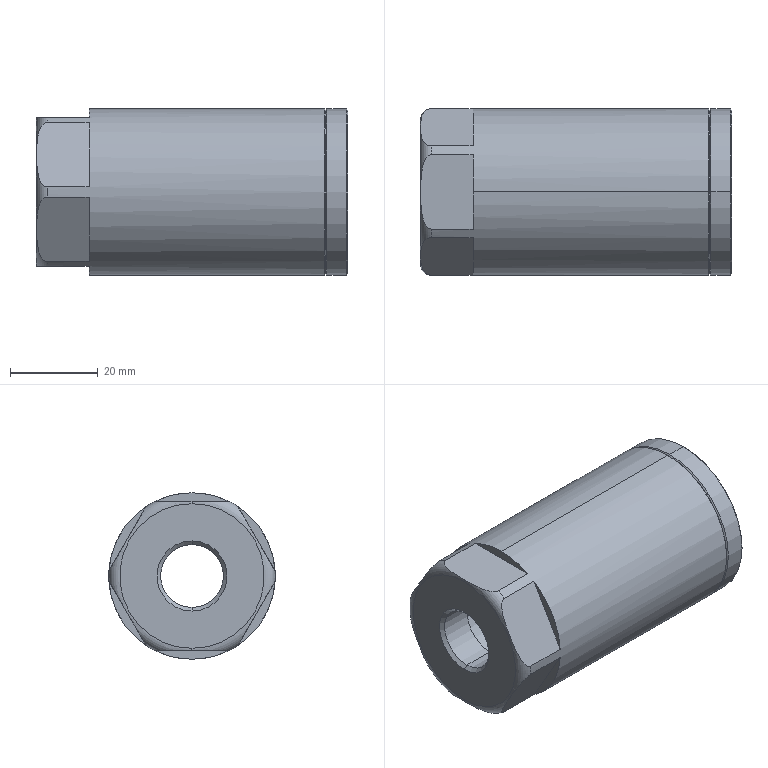Part | SolidWorks | features RefAxis 3, 3DProfileFeature 1, ICE 1, RevCut 1, Revolution 1 | 1 solid | 35 faces | box 71 x 38 x 38 mm | volume 56473 mm3 | plane 15 | cone 10 | cylinder 8 | torus 2 | commonest cylinder face diameters 14.376 x2 20.7 x2 37.9 x2 38 x2
STEP:
#1=CARTESIAN_POINT('',(71.,0.,-10.35));
#2=VERTEX_POINT('',#1);
#3=CARTESIAN_POINT('',(71.,0.,10.35));
#4=VERTEX_POINT('',#3);
#5=CARTESIAN_POINT('',(71.,0.,0.));
#6=DIRECTION('',(-1.,0.,0.));
#7=DIRECTION('',(0.,0.,1.));
#8=AXIS2_PLACEMENT_3D('',#5,#6,#7);
#9=CIRCLE('',#8,10.35);
#10=EDGE_CURVE('',#2,#4,#9,.T.);
#11=ORIENTED_EDGE('',*,*,#10,.F.);
#12=CARTESIAN_POINT('',(10.,0.,-10.35));
#13=VERTEX_POINT('',#12);
#14=CARTESIAN_POINT('',(71.,0.,-10.35));
#15=DIRECTION('',(-1.,0.,0.));
#16=VECTOR('',#15,1000.);
#17=LINE('',#14,#16);
#18=EDGE_CURVE('',#2,#13,#17,.T.);
#19=ORIENTED_EDGE('',*,*,#18,.T.);
#20=CARTESIAN_POINT('',(10.,0.,10.35));
#21=VERTEX_POINT('',#20);
#22=CARTESIAN_POINT('',(10.,0.,0.));
#23=DIRECTION('',(-1.,0.,0.));
#24=DIRECTION('',(0.,0.,1.));
#25=AXIS2_PLACEMENT_3D('',#22,#23,#24);
#26=CIRCLE('',#25,10.35);
#27=EDGE_CURVE('',#13,#21,#26,.T.);
#28=ORIENTED_EDGE('',*,*,#27,.T.);
#29=CARTESIAN_POINT('',(71.,0.,10.35));
#30=DIRECTION('',(-1.,0.,0.));
#31=VECTOR('',#30,1000.);
#32=LINE('',#29,#31);
#33=EDGE_CURVE('',#4,#21,#32,.T.);
#34=ORIENTED_EDGE('',*,*,#33,.F.);
#35=EDGE_LOOP('',(#11,#19,#28,#34));
#36=FACE_OUTER_BOUND('',#35,.T.);
#37=CARTESIAN_POINT('',(71.,0.,0.));
#38=DIRECTION('',(-1.,0.,0.));
#39=DIRECTION('',(0.,0.,1.));
#40=AXIS2_PLACEMENT_3D('',#37,#38,#39);
#41=CYLINDRICAL_SURFACE('',#40,10.35);
#42=ADVANCED_FACE('',(#36),#41,.F.);
#43=CARTESIAN_POINT('',(8.174,0.,-7.188));
#44=VERTEX_POINT('',#43);
#45=CARTESIAN_POINT('',(8.174,0.,7.188));
#46=VERTEX_POINT('',#45);
#47=CARTESIAN_POINT('',(8.174,0.,0.));
#48=DIRECTION('',(-1.,0.,0.));
#49=DIRECTION('',(0.,0.,1.));
#50=AXIS2_PLACEMENT_3D('',#47,#48,#49);
#51=CIRCLE('',#50,7.188);
#52=EDGE_CURVE('',#44,#46,#51,.T.);
#53=ORIENTED_EDGE('',*,*,#52,.T.);
#54=CARTESIAN_POINT('',(10.,0.,10.35));
#55=DIRECTION('',(0.5,0.,0.866));
#56=VECTOR('',#55,1000.);
#57=LINE('',#54,#56);
#58=EDGE_CURVE('',#46,#21,#57,.T.);
#59=ORIENTED_EDGE('',*,*,#58,.T.);
#60=ORIENTED_EDGE('',*,*,#27,.F.);
#61=CARTESIAN_POINT('',(10.,0.,-10.35));
#62=DIRECTION('',(0.5,0.,-0.866));
#63=VECTOR('',#62,1000.);
#64=LINE('',#61,#63);
#65=EDGE_CURVE('',#44,#13,#64,.T.);
#66=ORIENTED_EDGE('',*,*,#65,.F.);
#67=EDGE_LOOP('',(#53,#59,#60,#66));
#68=FACE_OUTER_BOUND('',#67,.T.);
#69=CARTESIAN_POINT('',(10.,0.,0.));
#70=DIRECTION('',(1.,0.,0.));
#71=DIRECTION('',(0.,0.,-1.));
#72=AXIS2_PLACEMENT_3D('',#69,#70,#71);
#73=CONICAL_SURFACE('',#72,10.35,1.047);
#74=ADVANCED_FACE('',(#68),#73,.F.);
#75=ORIENTED_EDGE('',*,*,#52,.F.);
#76=CARTESIAN_POINT('',(0.812,0.,-7.188));
#77=VERTEX_POINT('',#76);
#78=CARTESIAN_POINT('',(71.,0.,-7.188));
#79=DIRECTION('',(-1.,0.,0.));
#80=VECTOR('',#79,1000.);
#81=LINE('',#78,#80);
#82=EDGE_CURVE('',#44,#77,#81,.T.);
#83=ORIENTED_EDGE('',*,*,#82,.T.);
#84=CARTESIAN_POINT('',(0.812,0.,7.188));
#85=VERTEX_POINT('',#84);
#86=CARTESIAN_POINT('',(0.812,0.,0.));
#87=DIRECTION('',(-1.,0.,0.));
#88=DIRECTION('',(0.,0.,1.));
#89=AXIS2_PLACEMENT_3D('',#86,#87,#88);
#90=CIRCLE('',#89,7.188);
#91=EDGE_CURVE('',#77,#85,#90,.T.);
#92=ORIENTED_EDGE('',*,*,#91,.T.);
#93=CARTESIAN_POINT('',(71.,0.,7.188));
#94=DIRECTION('',(-1.,0.,0.));
#95=VECTOR('',#94,1000.);
#96=LINE('',#93,#95);
#97=EDGE_CURVE('',#46,#85,#96,.T.);
#98=ORIENTED_EDGE('',*,*,#97,.F.);
#99=EDGE_LOOP('',(#75,#83,#92,#98));
#100=FACE_OUTER_BOUND('',#99,.T.);
#101=CARTESIAN_POINT('',(71.,0.,0.));
#102=DIRECTION('',(-1.,0.,0.));
#103=DIRECTION('',(0.,0.,1.));
#104=AXIS2_PLACEMENT_3D('',#101,#102,#103);
#105=CYLINDRICAL_SURFACE('',#104,7.188);
#106=ADVANCED_FACE('',(#100),#105,.F.);
#107=ORIENTED_EDGE('',*,*,#91,.F.);
#108=CARTESIAN_POINT('',(0.,0.,-8.));
#109=VERTEX_POINT('',#108);
#110=CARTESIAN_POINT('',(0.812,0.,-7.188));
#111=DIRECTION('',(-0.7071,0.,-0.7071));
#112=VECTOR('',#111,1000.);
#113=LINE('',#110,#112);
#114=EDGE_CURVE('',#77,#109,#113,.T.);
#115=ORIENTED_EDGE('',*,*,#114,.T.);
#116=CARTESIAN_POINT('',(0.,0.,8.));
#117=VERTEX_POINT('',#116);
#118=CARTESIAN_POINT('',(0.,0.,0.));
#119=DIRECTION('',(-1.,0.,0.));
#120=DIRECTION('',(0.,0.,1.));
#121=AXIS2_PLACEMENT_3D('',#118,#119,#120);
#122=CIRCLE('',#121,8.);
#123=EDGE_CURVE('',#109,#117,#122,.T.);
#124=ORIENTED_EDGE('',*,*,#123,.T.);
#125=CARTESIAN_POINT('',(0.812,0.,7.188));
#126=DIRECTION('',(-0.7071,0.,0.7071));
#127=VECTOR('',#126,1000.);
#128=LINE('',#125,#127);
#129=EDGE_CURVE('',#85,#117,#128,.T.);
#130=ORIENTED_EDGE('',*,*,#129,.F.);
#131=EDGE_LOOP('',(#107,#115,#124,#130));
#132=FACE_OUTER_BOUND('',#131,.T.);
#133=CARTESIAN_POINT('',(0.812,0.,0.));
#134=DIRECTION('',(-1.,0.,0.));
#135=DIRECTION('',(0.,0.,1.));
#136=AXIS2_PLACEMENT_3D('',#133,#134,#135);
#137=CONICAL_SURFACE('',#136,7.188,0.7854);
#138=ADVANCED_FACE('',(#132),#137,.F.);
#139=CARTESIAN_POINT('',(71.,0.,18.65));
#140=VERTEX_POINT('',#139);
#141=CARTESIAN_POINT('',(71.,0.,-18.65));
#142=VERTEX_POINT('',#141);
#143=CARTESIAN_POINT('',(71.,0.,0.));
#144=DIRECTION('',(-1.,0.,0.));
#145=DIRECTION('',(0.,0.,1.));
#146=AXIS2_PLACEMENT_3D('',#143,#144,#145);
#147=CIRCLE('',#146,18.65);
#148=EDGE_CURVE('',#140,#142,#147,.T.);
#149=ORIENTED_EDGE('',*,*,#148,.T.);
#150=CARTESIAN_POINT('',(70.7,0.,-18.95));
#151=VERTEX_POINT('',#150);
#152=CARTESIAN_POINT('',(71.,0.,-18.65));
#153=DIRECTION('',(-0.7071,0.,-0.7071));
#154=VECTOR('',#153,1000.);
#155=LINE('',#152,#154);
#156=EDGE_CURVE('',#142,#151,#155,.T.);
#157=ORIENTED_EDGE('',*,*,#156,.T.);
#158=CARTESIAN_POINT('',(70.7,0.,18.95));
#159=VERTEX_POINT('',#158);
#160=CARTESIAN_POINT('',(70.7,0.,0.));
#161=DIRECTION('',(-1.,0.,0.));
#162=DIRECTION('',(0.,0.,1.));
#163=AXIS2_PLACEMENT_3D('',#160,#161,#162);
#164=CIRCLE('',#163,18.95);
#165=EDGE_CURVE('',#159,#151,#164,.T.);
#166=ORIENTED_EDGE('',*,*,#165,.F.);
#167=CARTESIAN_POINT('',(71.,0.,18.65));
#168=DIRECTION('',(-0.7071,0.,0.7071));
#169=VECTOR('',#168,1000.);
#170=LINE('',#167,#169);
#171=EDGE_CURVE('',#140,#159,#170,.T.);
#172=ORIENTED_EDGE('',*,*,#171,.F.);
#173=EDGE_LOOP('',(#149,#157,#166,#172));
#174=FACE_OUTER_BOUND('',#173,.T.);
#175=CARTESIAN_POINT('',(71.,0.,0.));
#176=DIRECTION('',(-1.,0.,0.));
#177=DIRECTION('',(0.,0.,1.));
#178=AXIS2_PLACEMENT_3D('',#175,#176,#177);
#179=CONICAL_SURFACE('',#178,18.65,0.7854);
#180=ADVANCED_FACE('',(#174),#179,.T.);
#181=ORIENTED_EDGE('',*,*,#165,.T.);
#182=CARTESIAN_POINT('',(66.3,0.,-18.95));
#183=VERTEX_POINT('',#182);
#184=CARTESIAN_POINT('',(71.,0.,-18.95));
#185=DIRECTION('',(-1.,0.,0.));
#186=VECTOR('',#185,1000.);
#187=LINE('',#184,#186);
#188=EDGE_CURVE('',#151,#183,#187,.T.);
#189=ORIENTED_EDGE('',*,*,#188,.T.);
#190=CARTESIAN_POINT('',(66.3,0.,18.95));
#191=VERTEX_POINT('',#190);
#192=CARTESIAN_POINT('',(66.3,0.,0.));
#193=DIRECTION('',(-1.,0.,0.));
#194=DIRECTION('',(0.,0.,1.));
#195=AXIS2_PLACEMENT_3D('',#192,#193,#194);
#196=CIRCLE('',#195,18.95);
#197=EDGE_CURVE('',#191,#183,#196,.T.);
#198=ORIENTED_EDGE('',*,*,#197,.F.);
#199=CARTESIAN_POINT('',(71.,0.,18.95));
#200=DIRECTION('',(-1.,0.,0.));
#201=VECTOR('',#200,1000.);
#202=LINE('',#199,#201);
#203=EDGE_CURVE('',#159,#191,#202,.T.);
#204=ORIENTED_EDGE('',*,*,#203,.F.);
#205=EDGE_LOOP('',(#181,#189,#198,#204));
#206=FACE_OUTER_BOUND('',#205,.T.);
#207=CARTESIAN_POINT('',(71.,0.,0.));
#208=DIRECTION('',(-1.,0.,0.));
#209=DIRECTION('',(0.,0.,1.));
#210=AXIS2_PLACEMENT_3D('',#207,#208,#209);
#211=CYLINDRICAL_SURFACE('',#210,18.95);
#212=ADVANCED_FACE('',(#206),#211,.T.);
#213=CARTESIAN_POINT('',(66.,0.,18.65));
#214=VERTEX_POINT('',#213);
#215=CARTESIAN_POINT('',(66.,0.,-18.65));
#216=VERTEX_POINT('',#215);
#217=CARTESIAN_POINT('',(66.,0.,0.));
#218=DIRECTION('',(-1.,0.,0.));
#219=DIRECTION('',(0.,0.,1.));
#220=AXIS2_PLACEMENT_3D('',#217,#218,#219);
#221=CIRCLE('',#220,18.65);
#222=EDGE_CURVE('',#214,#216,#221,.T.);
#223=ORIENTED_EDGE('',*,*,#222,.F.);
#224=CARTESIAN_POINT('',(66.3,0.,18.95));
#225=DIRECTION('',(0.7071,0.,0.7071));
#226=VECTOR('',#225,1000.);
#227=LINE('',#224,#226);
#228=EDGE_CURVE('',#214,#191,#227,.T.);
#229=ORIENTED_EDGE('',*,*,#228,.T.);
#230=ORIENTED_EDGE('',*,*,#197,.T.);
#231=CARTESIAN_POINT('',(66.3,0.,-18.95));
#232=DIRECTION('',(0.7071,0.,-0.7071));
#233=VECTOR('',#232,1000.);
#234=LINE('',#231,#233);
#235=EDGE_CURVE('',#216,#183,#234,.T.);
#236=ORIENTED_EDGE('',*,*,#235,.F.);
#237=EDGE_LOOP('',(#223,#229,#230,#236));
#238=FACE_OUTER_BOUND('',#237,.T.);
#239=CARTESIAN_POINT('',(66.3,0.,0.));
#240=DIRECTION('',(1.,0.,0.));
#241=DIRECTION('',(0.,0.,-1.));
#242=AXIS2_PLACEMENT_3D('',#239,#240,#241);
#243=CONICAL_SURFACE('',#242,18.95,0.7854);
#244=ADVANCED_FACE('',(#238),#243,.T.);
#245=CARTESIAN_POINT('',(66.,0.,18.7));
#246=VERTEX_POINT('',#245);
#247=CARTESIAN_POINT('',(66.,0.,-18.7));
#248=VERTEX_POINT('',#247);
#249=CARTESIAN_POINT('',(66.,0.,0.));
#250=DIRECTION('',(-1.,0.,0.));
#251=DIRECTION('',(0.,0.,1.));
#252=AXIS2_PLACEMENT_3D('',#249,#250,#251);
#253=CIRCLE('',#252,18.7);
#254=EDGE_CURVE('',#246,#248,#253,.T.);
#255=ORIENTED_EDGE('',*,*,#254,.T.);
#256=CARTESIAN_POINT('',(65.7,0.,-19.));
#257=VERTEX_POINT('',#256);
#258=CARTESIAN_POINT('',(66.,0.,-18.7));
#259=DIRECTION('',(-0.7071,0.,-0.7071));
#260=VECTOR('',#259,1000.);
#261=LINE('',#258,#260);
#262=EDGE_CURVE('',#248,#257,#261,.T.);
#263=ORIENTED_EDGE('',*,*,#262,.T.);
#264=CARTESIAN_POINT('',(65.7,0.,19.));
#265=VERTEX_POINT('',#264);
#266=CARTESIAN_POINT('',(65.7,0.,0.));
#267=DIRECTION('',(-1.,0.,0.));
#268=DIRECTION('',(0.,0.,1.));
#269=AXIS2_PLACEMENT_3D('',#266,#267,#268);
#270=CIRCLE('',#269,19.);
#271=EDGE_CURVE('',#265,#257,#270,.T.);
#272=ORIENTED_EDGE('',*,*,#271,.F.);
#273=CARTESIAN_POINT('',(66.,0.,18.7));
#274=DIRECTION('',(-0.7071,0.,0.7071));
#275=VECTOR('',#274,1000.);
#276=LINE('',#273,#275);
#277=EDGE_CURVE('',#246,#265,#276,.T.);
#278=ORIENTED_EDGE('',*,*,#277,.F.);
#279=EDGE_LOOP('',(#255,#263,#272,#278));
#280=FACE_OUTER_BOUND('',#279,.T.);
#281=CARTESIAN_POINT('',(66.,0.,0.));
#282=DIRECTION('',(-1.,0.,0.));
#283=DIRECTION('',(0.,0.,1.));
#284=AXIS2_PLACEMENT_3D('',#281,#282,#283);
#285=CONICAL_SURFACE('',#284,18.7,0.7854);
#286=ADVANCED_FACE('',(#280),#285,.T.);
#287=ORIENTED_EDGE('',*,*,#271,.T.);
#288=CARTESIAN_POINT('',(12.,0.,-19.));
#289=VERTEX_POINT('',#288);
#290=CARTESIAN_POINT('',(71.,0.,-19.));
#291=DIRECTION('',(-1.,0.,0.));
#292=VECTOR('',#291,1000.);
#293=LINE('',#290,#292);
#294=EDGE_CURVE('',#257,#289,#293,.T.);
#295=ORIENTED_EDGE('',*,*,#294,.T.);
#296=CARTESIAN_POINT('',(12.,8.485,-17.));
#297=VERTEX_POINT('',#296);
#298=CARTESIAN_POINT('',(12.,0.,0.));
#299=DIRECTION('',(1.,0.,0.));
#300=DIRECTION('',(0.,0.,-1.));
#301=AXIS2_PLACEMENT_3D('',#298,#299,#300);
#302=CIRCLE('',#301,19.);
#303=EDGE_CURVE('',#289,#297,#302,.T.);
#304=ORIENTED_EDGE('',*,*,#303,.T.);
#305=CARTESIAN_POINT('',(2.5,8.485,-17.));
#306=VERTEX_POINT('',#305);
#307=CARTESIAN_POINT('',(71.,8.485,-17.));
#308=DIRECTION('',(-1.,0.,0.));
#309=VECTOR('',#308,1000.);
#310=LINE('',#307,#309);
#311=EDGE_CURVE('',#297,#306,#310,.T.);
#312=ORIENTED_EDGE('',*,*,#311,.T.);
#313=CARTESIAN_POINT('',(2.5,10.48,-15.848));
#314=VERTEX_POINT('',#313);
#315=CARTESIAN_POINT('',(2.5,0.,0.));
#316=DIRECTION('',(-1.,0.,0.));
#317=DIRECTION('',(0.,0.,1.));
#318=AXIS2_PLACEMENT_3D('',#315,#316,#317);
#319=CIRCLE('',#318,19.);
#320=EDGE_CURVE('',#314,#306,#319,.T.);
#321=ORIENTED_EDGE('',*,*,#320,.F.);
#322=CARTESIAN_POINT('',(12.,10.48,-15.848));
#323=VERTEX_POINT('',#322);
#324=CARTESIAN_POINT('',(71.,10.48,-15.848));
#325=DIRECTION('',(1.,0.,0.));
#326=VECTOR('',#325,1000.);
#327=LINE('',#324,#326);
#328=EDGE_CURVE('',#314,#323,#327,.T.);
#329=ORIENTED_EDGE('',*,*,#328,.T.);
#330=CARTESIAN_POINT('',(12.,18.965,-1.152));
#331=VERTEX_POINT('',#330);
#332=CARTESIAN_POINT('',(12.,0.,0.));
#333=DIRECTION('',(1.,0.,0.));
#334=DIRECTION('',(0.,0.,-1.));
#335=AXIS2_PLACEMENT_3D('',#332,#333,#334);
#336=CIRCLE('',#335,19.);
#337=EDGE_CURVE('',#323,#331,#336,.T.);
#338=ORIENTED_EDGE('',*,*,#337,.T.);
#339=CARTESIAN_POINT('',(2.5,18.965,-1.152));
#340=VERTEX_POINT('',#339);
#341=CARTESIAN_POINT('',(71.,18.965,-1.152));
#342=DIRECTION('',(-1.,0.,0.));
#343=VECTOR('',#342,1000.);
#344=LINE('',#341,#343);
#345=EDGE_CURVE('',#331,#340,#344,.T.);
#346=ORIENTED_EDGE('',*,*,#345,.T.);
#347=CARTESIAN_POINT('',(2.5,18.965,1.152));
#348=VERTEX_POINT('',#347);
#349=CARTESIAN_POINT('',(2.5,0.,0.));
#350=DIRECTION('',(-1.,0.,0.));
#351=DIRECTION('',(0.,0.,1.));
#352=AXIS2_PLACEMENT_3D('',#349,#350,#351);
#353=CIRCLE('',#352,19.);
#354=EDGE_CURVE('',#348,#340,#353,.T.);
#355=ORIENTED_EDGE('',*,*,#354,.F.);
#356=CARTESIAN_POINT('',(12.,18.965,1.152));
#357=VERTEX_POINT('',#356);
#358=CARTESIAN_POINT('',(71.,18.965,1.152));
#359=DIRECTION('',(1.,0.,0.));
#360=VECTOR('',#359,1000.);
#361=LINE('',#358,#360);
#362=EDGE_CURVE('',#348,#357,#361,.T.);
#363=ORIENTED_EDGE('',*,*,#362,.T.);
#364=CARTESIAN_POINT('',(12.,10.48,15.848));
#365=VERTEX_POINT('',#364);
#366=CARTESIAN_POINT('',(12.,0.,0.));
#367=DIRECTION('',(1.,0.,0.));
#368=DIRECTION('',(0.,0.,-1.));
#369=AXIS2_PLACEMENT_3D('',#366,#367,#368);
#370=CIRCLE('',#369,19.);
#371=EDGE_CURVE('',#357,#365,#370,.T.);
#372=ORIENTED_EDGE('',*,*,#371,.T.);
#373=CARTESIAN_POINT('',(2.5,10.48,15.848));
#374=VERTEX_POINT('',#373);
#375=CARTESIAN_POINT('',(71.,10.48,15.848));
#376=DIRECTION('',(-1.,0.,0.));
#377=VECTOR('',#376,1000.);
#378=LINE('',#375,#377);
#379=EDGE_CURVE('',#365,#374,#378,.T.);
#380=ORIENTED_EDGE('',*,*,#379,.T.);
#381=CARTESIAN_POINT('',(2.5,8.485,17.));
#382=VERTEX_POINT('',#381);
#383=CARTESIAN_POINT('',(2.5,0.,0.));
#384=DIRECTION('',(-1.,0.,0.));
#385=DIRECTION('',(0.,0.,1.));
#386=AXIS2_PLACEMENT_3D('',#383,#384,#385);
#387=CIRCLE('',#386,19.);
#388=EDGE_CURVE('',#382,#374,#387,.T.);
#389=ORIENTED_EDGE('',*,*,#388,.F.);
#390=CARTESIAN_POINT('',(12.,8.485,17.));
#391=VERTEX_POINT('',#390);
#392=CARTESIAN_POINT('',(71.,8.485,17.));
#393=DIRECTION('',(1.,0.,0.));
#394=VECTOR('',#393,1000.);
#395=LINE('',#392,#394);
#396=EDGE_CURVE('',#382,#391,#395,.T.);
#397=ORIENTED_EDGE('',*,*,#396,.T.);
#398=CARTESIAN_POINT('',(12.,0.,19.));
#399=VERTEX_POINT('',#398);
#400=CARTESIAN_POINT('',(12.,0.,0.));
#401=DIRECTION('',(1.,0.,0.));
#402=DIRECTION('',(0.,0.,-1.));
#403=AXIS2_PLACEMENT_3D('',#400,#401,#402);
#404=CIRCLE('',#403,19.);
#405=EDGE_CURVE('',#391,#399,#404,.T.);
#406=ORIENTED_EDGE('',*,*,#405,.T.);
#407=CARTESIAN_POINT('',(71.,0.,19.));
#408=DIRECTION('',(-1.,0.,0.));
#409=VECTOR('',#408,1000.);
#410=LINE('',#407,#409);
#411=EDGE_CURVE('',#265,#399,#410,.T.);
#412=ORIENTED_EDGE('',*,*,#411,.F.);
#413=EDGE_LOOP('',(#287,#295,#304,#312,#321,#329,#338,#346,#355,#363,#372,#380,#389,#397,#406,#412));
#414=FACE_OUTER_BOUND('',#413,.T.);
#415=CARTESIAN_POINT('',(71.,0.,0.));
#416=DIRECTION('',(-1.,0.,0.));
#417=DIRECTION('',(0.,0.,1.));
#418=AXIS2_PLACEMENT_3D('',#415,#416,#417);
#419=CYLINDRICAL_SURFACE('',#418,19.);
#420=ADVANCED_FACE('',(#414),#419,.T.);
#421=CARTESIAN_POINT('',(0.05051,0.,-17.));
#422=VERTEX_POINT('',#421);
#423=CARTESIAN_POINT('',(2.5,8.485,-17.));
#424=CARTESIAN_POINT('',(2.401,8.485,-17.));
#425=CARTESIAN_POINT('',(2.301,8.472,-17.));
#426=CARTESIAN_POINT('',(2.109,8.421,-17.));
#427=CARTESIAN_POINT('',(2.017,8.383,-17.));
#428=CARTESIAN_POINT('',(1.753,8.242,-17.));
#429=CARTESIAN_POINT('',(1.599,8.115,-17.));
#430=CARTESIAN_POINT('',(1.329,7.824,-17.));
#431=CARTESIAN_POINT('',(1.214,7.664,-17.));
#432=CARTESIAN_POINT('',(1.01,7.327,-17.));
#433=CARTESIAN_POINT('',(0.9209,7.148,-17.));
#434=CARTESIAN_POINT('',(0.6885,6.606,-17.));
#435=CARTESIAN_POINT('',(0.5747,6.231,-17.));
#436=CARTESIAN_POINT('',(0.3922,5.465,-17.));
#437=CARTESIAN_POINT('',(0.3248,5.076,-17.));
#438=CARTESIAN_POINT('',(0.1671,3.911,-17.));
#439=CARTESIAN_POINT('',(0.1184,3.13,-17.));
#440=CARTESIAN_POINT('',(0.07442,1.958,-17.));
#441=CARTESIAN_POINT('',(0.06512,1.566,-17.));
#442=CARTESIAN_POINT('',(0.05316,0.7835,-17.));
#443=CARTESIAN_POINT('',(0.05051,0.3935,-17.));
#444=CARTESIAN_POINT('',(0.05051,0.,-17.));
#445=B_SPLINE_CURVE_WITH_KNOTS('',3,(#423,#424,#425,#426,#427,#428,#429,#430,#431,#432,#433,#434,#435,#436,#437,#438,#439,#440,#441,#442,#443,#444),.UNSPECIFIED.,.F.,.F.,(4,2,2,2,2,2,2,2,2,2,4),(0.02818,0.02848,0.02877,0.02936,0.02995,0.03054,0.03172,0.0329,0.03525,0.03643,0.03761),.UNSPECIFIED.);
#446=EDGE_CURVE('',#306,#422,#445,.T.);
#447=ORIENTED_EDGE('',*,*,#446,.T.);
#448=CARTESIAN_POINT('',(0.,0.,-16.5));
#449=VERTEX_POINT('',#448);
#450=CARTESIAN_POINT('',(2.5,0.,-16.5));
#451=DIRECTION('',(0.,1.,0.));
#452=DIRECTION('',(0.,0.,1.));
#453=AXIS2_PLACEMENT_3D('',#450,#451,#452);
#454=CIRCLE('',#453,2.5);
#455=EDGE_CURVE('',#422,#449,#454,.T.);
#456=ORIENTED_EDGE('',*,*,#455,.T.);
#457=CARTESIAN_POINT('',(0.,0.,16.5));
#458=VERTEX_POINT('',#457);
#459=CARTESIAN_POINT('',(0.,0.,0.));
#460=DIRECTION('',(-1.,0.,0.));
#461=DIRECTION('',(0.,0.,1.));
#462=AXIS2_PLACEMENT_3D('',#459,#460,#461);
#463=CIRCLE('',#462,16.5);
#464=EDGE_CURVE('',#458,#449,#463,.T.);
#465=ORIENTED_EDGE('',*,*,#464,.F.);
#466=CARTESIAN_POINT('',(0.05051,0.,17.));
#467=VERTEX_POINT('',#466);
#468=CARTESIAN_POINT('',(2.5,0.,16.5));
#469=DIRECTION('',(0.,-1.,0.));
#470=DIRECTION('',(0.,0.,-1.));
#471=AXIS2_PLACEMENT_3D('',#468,#469,#470);
#472=CIRCLE('',#471,2.5);
#473=EDGE_CURVE('',#467,#458,#472,.T.);
#474=ORIENTED_EDGE('',*,*,#473,.F.);
#475=CARTESIAN_POINT('',(0.05051,0.,17.));
#476=CARTESIAN_POINT('',(0.05051,0.7839,17.));
#477=CARTESIAN_POINT('',(0.05974,1.567,17.));
#478=CARTESIAN_POINT('',(0.1185,3.132,17.));
#479=CARTESIAN_POINT('',(0.1672,3.913,17.));
#480=CARTESIAN_POINT('',(0.3256,5.081,17.));
#481=CARTESIAN_POINT('',(0.3931,5.469,17.));
#482=CARTESIAN_POINT('',(0.5742,6.228,17.));
#483=CARTESIAN_POINT('',(0.687,6.601,17.));
#484=CARTESIAN_POINT('',(0.9946,7.321,17.));
#485=CARTESIAN_POINT('',(1.191,7.675,17.));
#486=CARTESIAN_POINT('',(1.597,8.113,17.));
#487=CARTESIAN_POINT('',(1.751,8.241,17.));
#488=CARTESIAN_POINT('',(2.016,8.383,17.));
#489=CARTESIAN_POINT('',(2.108,8.42,17.));
#490=CARTESIAN_POINT('',(2.3,8.472,17.));
#491=CARTESIAN_POINT('',(2.401,8.485,17.));
#492=CARTESIAN_POINT('',(2.5,8.485,17.));
#493=B_SPLINE_CURVE_WITH_KNOTS('',3,(#475,#476,#477,#478,#479,#480,#481,#482,#483,#484,#485,#486,#487,#488,#489,#490,#491,#492),.UNSPECIFIED.,.F.,.F.,(4,2,2,2,2,2,2,2,4),(0.,0.002348,0.004697,0.005871,0.007045,0.00822,0.008807,0.0091,0.009394),.UNSPECIFIED.);
#494=EDGE_CURVE('',#467,#382,#493,.T.);
#495=ORIENTED_EDGE('',*,*,#494,.T.);
#496=ORIENTED_EDGE('',*,*,#388,.T.);
#497=CARTESIAN_POINT('',(2.5,10.48,15.848));
#498=CARTESIAN_POINT('',(2.399,10.48,15.848));
#499=CARTESIAN_POINT('',(2.301,10.487,15.837));
#500=CARTESIAN_POINT('',(2.109,10.512,15.792));
#501=CARTESIAN_POINT('',(2.016,10.531,15.759));
#502=CARTESIAN_POINT('',(1.753,10.601,15.638));
#503=CARTESIAN_POINT('',(1.597,10.666,15.526));
#504=CARTESIAN_POINT('',(1.328,10.811,15.275));
#505=CARTESIAN_POINT('',(1.211,10.892,15.134));
#506=CARTESIAN_POINT('',(1.007,11.062,14.841));
#507=CARTESIAN_POINT('',(0.9196,11.15,14.688));
#508=CARTESIAN_POINT('',(0.7645,11.331,14.374));
#509=CARTESIAN_POINT('',(0.6967,11.425,14.212));
#510=CARTESIAN_POINT('',(0.5779,11.613,13.886));
#511=CARTESIAN_POINT('',(0.5267,11.707,13.722));
#512=CARTESIAN_POINT('',(0.3911,11.993,13.227));
#513=CARTESIAN_POINT('',(0.3245,12.185,12.894));
#514=CARTESIAN_POINT('',(0.1674,12.766,11.889));
#515=CARTESIAN_POINT('',(0.1183,13.158,11.21));
#516=CARTESIAN_POINT('',(0.05959,13.942,9.852));
#517=CARTESIAN_POINT('',(0.05043,14.334,9.172));
#518=CARTESIAN_POINT('',(0.05059,15.119,7.813));
#519=CARTESIAN_POINT('',(0.05991,15.511,7.134));
#520=CARTESIAN_POINT('',(0.1193,16.295,5.775));
#521=CARTESIAN_POINT('',(0.1687,16.688,5.096));
#522=CARTESIAN_POINT('',(0.3281,17.271,4.086));
#523=CARTESIAN_POINT('',(0.396,17.464,3.751));
#524=CARTESIAN_POINT('',(0.5785,17.844,3.093));
#525=CARTESIAN_POINT('',(0.6924,18.031,2.769));
#526=CARTESIAN_POINT('',(0.9268,18.303,2.299));
#527=CARTESIAN_POINT('',(1.015,18.391,2.146));
#528=CARTESIAN_POINT('',(1.22,18.559,1.855));
#529=CARTESIAN_POINT('',(1.336,18.639,1.716));
#530=CARTESIAN_POINT('',(1.604,18.782,1.469));
#531=CARTESIAN_POINT('',(1.759,18.846,1.358));
#532=CARTESIAN_POINT('',(2.02,18.915,1.239));
#533=CARTESIAN_POINT('',(2.113,18.933,1.206));
#534=CARTESIAN_POINT('',(2.303,18.958,1.163));
#535=CARTESIAN_POINT('',(2.4,18.965,1.152));
#536=CARTESIAN_POINT('',(2.5,18.965,1.152));
#537=B_SPLINE_CURVE_WITH_KNOTS('',3,(#497,#498,#499,#500,#501,#502,#503,#504,#505,#506,#507,#508,#509,#510,#511,#512,#513,#514,#515,#516,#517,#518,#519,#520,#521,#522,#523,#524,#525,#526,#527,#528,#529,#530,#531,#532,#533,#534,#535,#536),.UNSPECIFIED.,.F.,.F.,(4,2,2,2,2,2,2,2,2,2,2,2,2,2,2,2,2,2,2,4),(0.000000197,0.0002971,0.000594,0.001188,0.001781,0.002375,0.002969,0.003563,0.00475,0.007125,0.0095,0.01188,0.01425,0.01544,0.01663,0.01722,0.01781,0.01841,0.0187,0.019),.UNSPECIFIED.);
#538=EDGE_CURVE('',#374,#348,#537,.T.);
#539=ORIENTED_EDGE('',*,*,#538,.T.);
#540=ORIENTED_EDGE('',*,*,#354,.T.);
#541=CARTESIAN_POINT('',(2.5,18.965,-1.152));
#542=CARTESIAN_POINT('',(2.399,18.965,-1.152));
#543=CARTESIAN_POINT('',(2.301,18.958,-1.163));
#544=CARTESIAN_POINT('',(2.109,18.933,-1.208));
#545=CARTESIAN_POINT('',(2.016,18.914,-1.241));
#546=CARTESIAN_POINT('',(1.753,18.844,-1.362));
#547=CARTESIAN_POINT('',(1.597,18.779,-1.474));
#548=CARTESIAN_POINT('',(1.328,18.634,-1.725));
#549=CARTESIAN_POINT('',(1.211,18.552,-1.866));
#550=CARTESIAN_POINT('',(1.007,18.383,-2.159));
#551=CARTESIAN_POINT('',(0.9196,18.295,-2.312));
#552=CARTESIAN_POINT('',(0.7645,18.114,-2.626));
#553=CARTESIAN_POINT('',(0.6967,18.02,-2.788));
#554=CARTESIAN_POINT('',(0.5779,17.832,-3.114));
#555=CARTESIAN_POINT('',(0.5267,17.737,-3.278));
#556=CARTESIAN_POINT('',(0.3911,17.452,-3.773));
#557=CARTESIAN_POINT('',(0.3245,17.259,-4.106));
#558=CARTESIAN_POINT('',(0.1674,16.679,-5.111));
#559=CARTESIAN_POINT('',(0.1183,16.287,-5.79));
#560=CARTESIAN_POINT('',(0.05959,15.503,-7.148));
#561=CARTESIAN_POINT('',(0.05043,15.111,-7.828));
#562=CARTESIAN_POINT('',(0.05059,14.326,-9.187));
#563=CARTESIAN_POINT('',(0.05991,13.933,-9.866));
#564=CARTESIAN_POINT('',(0.1193,13.149,-11.225));
#565=CARTESIAN_POINT('',(0.1687,12.757,-11.904));
#566=CARTESIAN_POINT('',(0.3281,12.174,-12.914));
#567=CARTESIAN_POINT('',(0.396,11.981,-13.249));
#568=CARTESIAN_POINT('',(0.5785,11.601,-13.907));
#569=CARTESIAN_POINT('',(0.6924,11.414,-14.231));
#570=CARTESIAN_POINT('',(0.9268,11.142,-14.701));
#571=CARTESIAN_POINT('',(1.015,11.054,-14.854));
#572=CARTESIAN_POINT('',(1.22,10.886,-15.145));
#573=CARTESIAN_POINT('',(1.336,10.806,-15.284));
#574=CARTESIAN_POINT('',(1.604,10.663,-15.531));
#575=CARTESIAN_POINT('',(1.759,10.599,-15.642));
#576=CARTESIAN_POINT('',(2.02,10.53,-15.761));
#577=CARTESIAN_POINT('',(2.113,10.512,-15.794));
#578=CARTESIAN_POINT('',(2.303,10.486,-15.837));
#579=CARTESIAN_POINT('',(2.4,10.48,-15.848));
#580=CARTESIAN_POINT('',(2.5,10.48,-15.848));
#581=B_SPLINE_CURVE_WITH_KNOTS('',3,(#541,#542,#543,#544,#545,#546,#547,#548,#549,#550,#551,#552,#553,#554,#555,#556,#557,#558,#559,#560,#561,#562,#563,#564,#565,#566,#567,#568,#569,#570,#571,#572,#573,#574,#575,#576,#577,#578,#579,#580),.UNSPECIFIED.,.F.,.F.,(4,2,2,2,2,2,2,2,2,2,2,2,2,2,2,2,2,2,2,4),(0.000000197,0.0002971,0.000594,0.001188,0.001781,0.002375,0.002969,0.003563,0.00475,0.007125,0.0095,0.01188,0.01425,0.01544,0.01663,0.01722,0.01781,0.01841,0.0187,0.019),.UNSPECIFIED.);
#582=EDGE_CURVE('',#340,#314,#581,.T.);
#583=ORIENTED_EDGE('',*,*,#582,.T.);
#584=ORIENTED_EDGE('',*,*,#320,.T.);
#585=EDGE_LOOP('',(#447,#456,#465,#474,#495,#496,#539,#540,#583,#584));
#586=FACE_OUTER_BOUND('',#585,.T.);
#587=CARTESIAN_POINT('',(2.5,0.,0.));
#588=DIRECTION('',(-1.,0.,0.));
#589=DIRECTION('',(0.,0.,1.));
#590=AXIS2_PLACEMENT_3D('',#587,#588,#589);
#591=TOROIDAL_SURFACE('',#590,16.5,2.5);
#592=ADVANCED_FACE('',(#586),#591,.T.);
#593=CARTESIAN_POINT('',(0.,0.,0.));
#594=DIRECTION('',(-1.,0.,0.));
#595=DIRECTION('',(0.,0.,1.));
#596=AXIS2_PLACEMENT_3D('',#593,#594,#595);
#597=CIRCLE('',#596,8.);
#598=EDGE_CURVE('',#117,#109,#597,.T.);
#599=ORIENTED_EDGE('',*,*,#598,.F.);
#600=ORIENTED_EDGE('',*,*,#123,.F.);
#601=EDGE_LOOP('',(#599,#600));
#602=FACE_BOUND('',#601,.T.);
#603=ORIENTED_EDGE('',*,*,#464,.T.);
#604=CARTESIAN_POINT('',(0.,0.,0.));
#605=DIRECTION('',(-1.,0.,0.));
#606=DIRECTION('',(0.,0.,1.));
#607=AXIS2_PLACEMENT_3D('',#604,#605,#606);
#608=CIRCLE('',#607,16.5);
#609=EDGE_CURVE('',#449,#458,#608,.T.);
#610=ORIENTED_EDGE('',*,*,#609,.T.);
#611=EDGE_LOOP('',(#603,#610));
#612=FACE_OUTER_BOUND('',#611,.T.);
#613=CARTESIAN_POINT('',(0.,0.,0.));
#614=DIRECTION('',(1.,0.,0.));
#615=DIRECTION('',(0.,0.,-1.));
#616=AXIS2_PLACEMENT_3D('',#613,#614,#615);
#617=PLANE('',#616);
#618=ADVANCED_FACE('',(#602,#612),#617,.F.);
#619=ORIENTED_EDGE('',*,*,#455,.F.);
#620=CARTESIAN_POINT('',(2.5,-8.485,-17.));
#621=VERTEX_POINT('',#620);
#622=CARTESIAN_POINT('',(0.05051,0.,-17.));
#623=CARTESIAN_POINT('',(0.05051,-0.7839,-17.));
#624=CARTESIAN_POINT('',(0.05974,-1.567,-17.));
#625=CARTESIAN_POINT('',(0.1185,-3.132,-17.));
#626=CARTESIAN_POINT('',(0.1672,-3.913,-17.));
#627=CARTESIAN_POINT('',(0.3256,-5.081,-17.));
#628=CARTESIAN_POINT('',(0.3931,-5.469,-17.));
#629=CARTESIAN_POINT('',(0.5742,-6.228,-17.));
#630=CARTESIAN_POINT('',(0.687,-6.601,-17.));
#631=CARTESIAN_POINT('',(0.9946,-7.321,-17.));
#632=CARTESIAN_POINT('',(1.191,-7.675,-17.));
#633=CARTESIAN_POINT('',(1.597,-8.113,-17.));
#634=CARTESIAN_POINT('',(1.751,-8.241,-17.));
#635=CARTESIAN_POINT('',(2.016,-8.383,-17.));
#636=CARTESIAN_POINT('',(2.108,-8.42,-17.));
#637=CARTESIAN_POINT('',(2.3,-8.472,-17.));
#638=CARTESIAN_POINT('',(2.401,-8.485,-17.));
#639=CARTESIAN_POINT('',(2.5,-8.485,-17.));
#640=B_SPLINE_CURVE_WITH_KNOTS('',3,(#622,#623,#624,#625,#626,#627,#628,#629,#630,#631,#632,#633,#634,#635,#636,#637,#638,#639),.UNSPECIFIED.,.F.,.F.,(4,2,2,2,2,2,2,2,4),(0.,0.002348,0.004697,0.005871,0.007045,0.00822,0.008807,0.0091,0.009394),.UNSPECIFIED.);
#641=EDGE_CURVE('',#422,#621,#640,.T.);
#642=ORIENTED_EDGE('',*,*,#641,.T.);
#643=CARTESIAN_POINT('',(2.5,-10.48,-15.848));
#644=VERTEX_POINT('',#643);
#645=CARTESIAN_POINT('',(2.5,0.,0.));
#646=DIRECTION('',(-1.,0.,0.));
#647=DIRECTION('',(0.,0.,1.));
#648=AXIS2_PLACEMENT_3D('',#645,#646,#647);
#649=CIRCLE('',#648,19.);
#650=EDGE_CURVE('',#621,#644,#649,.T.);
#651=ORIENTED_EDGE('',*,*,#650,.T.);
#652=CARTESIAN_POINT('',(2.5,-18.965,-1.152));
#653=VERTEX_POINT('',#652);
#654=CARTESIAN_POINT('',(2.5,-10.48,-15.848));
#655=CARTESIAN_POINT('',(2.399,-10.48,-15.848));
#656=CARTESIAN_POINT('',(2.301,-10.487,-15.837));
#657=CARTESIAN_POINT('',(2.109,-10.512,-15.792));
#658=CARTESIAN_POINT('',(2.016,-10.531,-15.759));
#659=CARTESIAN_POINT('',(1.753,-10.601,-15.638));
#660=CARTESIAN_POINT('',(1.597,-10.666,-15.526));
#661=CARTESIAN_POINT('',(1.328,-10.811,-15.275));
#662=CARTESIAN_POINT('',(1.211,-10.892,-15.134));
#663=CARTESIAN_POINT('',(1.007,-11.062,-14.841));
#664=CARTESIAN_POINT('',(0.9196,-11.15,-14.688));
#665=CARTESIAN_POINT('',(0.7645,-11.331,-14.374));
#666=CARTESIAN_POINT('',(0.6967,-11.425,-14.212));
#667=CARTESIAN_POINT('',(0.5779,-11.613,-13.886));
#668=CARTESIAN_POINT('',(0.5267,-11.707,-13.722));
#669=CARTESIAN_POINT('',(0.3911,-11.993,-13.227));
#670=CARTESIAN_POINT('',(0.3245,-12.185,-12.894));
#671=CARTESIAN_POINT('',(0.1674,-12.766,-11.889));
#672=CARTESIAN_POINT('',(0.1183,-13.158,-11.21));
#673=CARTESIAN_POINT('',(0.05959,-13.942,-9.852));
#674=CARTESIAN_POINT('',(0.05043,-14.334,-9.172));
#675=CARTESIAN_POINT('',(0.05059,-15.119,-7.813));
#676=CARTESIAN_POINT('',(0.05991,-15.511,-7.134));
#677=CARTESIAN_POINT('',(0.1193,-16.295,-5.775));
#678=CARTESIAN_POINT('',(0.1687,-16.688,-5.096));
#679=CARTESIAN_POINT('',(0.3281,-17.271,-4.086));
#680=CARTESIAN_POINT('',(0.396,-17.464,-3.751));
#681=CARTESIAN_POINT('',(0.5785,-17.844,-3.093));
#682=CARTESIAN_POINT('',(0.6924,-18.031,-2.769));
#683=CARTESIAN_POINT('',(0.9268,-18.303,-2.299));
#684=CARTESIAN_POINT('',(1.015,-18.391,-2.146));
#685=CARTESIAN_POINT('',(1.22,-18.559,-1.855));
#686=CARTESIAN_POINT('',(1.336,-18.639,-1.716));
#687=CARTESIAN_POINT('',(1.604,-18.782,-1.469));
#688=CARTESIAN_POINT('',(1.759,-18.846,-1.358));
#689=CARTESIAN_POINT('',(2.02,-18.915,-1.239));
#690=CARTESIAN_POINT('',(2.113,-18.933,-1.206));
#691=CARTESIAN_POINT('',(2.303,-18.958,-1.163));
#692=CARTESIAN_POINT('',(2.4,-18.965,-1.152));
#693=CARTESIAN_POINT('',(2.5,-18.965,-1.152));
#694=B_SPLINE_CURVE_WITH_KNOTS('',3,(#654,#655,#656,#657,#658,#659,#660,#661,#662,#663,#664,#665,#666,#667,#668,#669,#670,#671,#672,#673,#674,#675,#676,#677,#678,#679,#680,#681,#682,#683,#684,#685,#686,#687,#688,#689,#690,#691,#692,#693),.UNSPECIFIED.,.F.,.F.,(4,2,2,2,2,2,2,2,2,2,2,2,2,2,2,2,2,2,2,4),(0.000000197,0.0002971,0.000594,0.001188,0.001781,0.002375,0.002969,0.003563,0.00475,0.007125,0.0095,0.01188,0.01425,0.01544,0.01663,0.01722,0.01781,0.01841,0.0187,0.019),.UNSPECIFIED.);
#695=EDGE_CURVE('',#644,#653,#694,.T.);
#696=ORIENTED_EDGE('',*,*,#695,.T.);
#697=CARTESIAN_POINT('',(2.5,-18.965,1.152));
#698=VERTEX_POINT('',#697);
#699=CARTESIAN_POINT('',(2.5,0.,0.));
#700=DIRECTION('',(-1.,0.,0.));
#701=DIRECTION('',(0.,0.,1.));
#702=AXIS2_PLACEMENT_3D('',#699,#700,#701);
#703=CIRCLE('',#702,19.);
#704=EDGE_CURVE('',#653,#698,#703,.T.);
#705=ORIENTED_EDGE('',*,*,#704,.T.);
#706=CARTESIAN_POINT('',(2.5,-10.48,15.848));
#707=VERTEX_POINT('',#706);
#708=CARTESIAN_POINT('',(2.5,-18.965,1.152));
#709=CARTESIAN_POINT('',(2.399,-18.965,1.152));
#710=CARTESIAN_POINT('',(2.301,-18.958,1.163));
#711=CARTESIAN_POINT('',(2.109,-18.933,1.208));
#712=CARTESIAN_POINT('',(2.016,-18.914,1.241));
#713=CARTESIAN_POINT('',(1.753,-18.844,1.362));
#714=CARTESIAN_POINT('',(1.597,-18.779,1.474));
#715=CARTESIAN_POINT('',(1.328,-18.634,1.725));
#716=CARTESIAN_POINT('',(1.211,-18.552,1.866));
#717=CARTESIAN_POINT('',(1.007,-18.383,2.159));
#718=CARTESIAN_POINT('',(0.9196,-18.295,2.312));
#719=CARTESIAN_POINT('',(0.7645,-18.114,2.626));
#720=CARTESIAN_POINT('',(0.6967,-18.02,2.788));
#721=CARTESIAN_POINT('',(0.5779,-17.832,3.114));
#722=CARTESIAN_POINT('',(0.5267,-17.737,3.278));
#723=CARTESIAN_POINT('',(0.3911,-17.452,3.773));
#724=CARTESIAN_POINT('',(0.3245,-17.259,4.106));
#725=CARTESIAN_POINT('',(0.1674,-16.679,5.111));
#726=CARTESIAN_POINT('',(0.1183,-16.287,5.79));
#727=CARTESIAN_POINT('',(0.05959,-15.503,7.148));
#728=CARTESIAN_POINT('',(0.05043,-15.111,7.828));
#729=CARTESIAN_POINT('',(0.05059,-14.326,9.187));
#730=CARTESIAN_POINT('',(0.05991,-13.933,9.866));
#731=CARTESIAN_POINT('',(0.1193,-13.149,11.225));
#732=CARTESIAN_POINT('',(0.1687,-12.757,11.904));
#733=CARTESIAN_POINT('',(0.3281,-12.174,12.914));
#734=CARTESIAN_POINT('',(0.396,-11.981,13.249));
#735=CARTESIAN_POINT('',(0.5785,-11.601,13.907));
#736=CARTESIAN_POINT('',(0.6924,-11.414,14.231));
#737=CARTESIAN_POINT('',(0.9268,-11.142,14.701));
#738=CARTESIAN_POINT('',(1.015,-11.054,14.854));
#739=CARTESIAN_POINT('',(1.22,-10.886,15.145));
#740=CARTESIAN_POINT('',(1.336,-10.806,15.284));
#741=CARTESIAN_POINT('',(1.604,-10.663,15.531));
#742=CARTESIAN_POINT('',(1.759,-10.599,15.642));
#743=CARTESIAN_POINT('',(2.02,-10.53,15.761));
#744=CARTESIAN_POINT('',(2.113,-10.512,15.794));
#745=CARTESIAN_POINT('',(2.303,-10.486,15.837));
#746=CARTESIAN_POINT('',(2.4,-10.48,15.848));
#747=CARTESIAN_POINT('',(2.5,-10.48,15.848));
#748=B_SPLINE_CURVE_WITH_KNOTS('',3,(#708,#709,#710,#711,#712,#713,#714,#715,#716,#717,#718,#719,#720,#721,#722,#723,#724,#725,#726,#727,#728,#729,#730,#731,#732,#733,#734,#735,#736,#737,#738,#739,#740,#741,#742,#743,#744,#745,#746,#747),.UNSPECIFIED.,.F.,.F.,(4,2,2,2,2,2,2,2,2,2,2,2,2,2,2,2,2,2,2,4),(0.000000197,0.0002971,0.000594,0.001188,0.001781,0.002375,0.002969,0.003563,0.00475,0.007125,0.0095,0.01188,0.01425,0.01544,0.01663,0.01722,0.01781,0.01841,0.0187,0.019),.UNSPECIFIED.);
#749=EDGE_CURVE('',#698,#707,#748,.T.);
#750=ORIENTED_EDGE('',*,*,#749,.T.);
#751=CARTESIAN_POINT('',(2.5,-8.485,17.));
#752=VERTEX_POINT('',#751);
#753=CARTESIAN_POINT('',(2.5,0.,0.));
#754=DIRECTION('',(-1.,0.,0.));
#755=DIRECTION('',(0.,0.,1.));
#756=AXIS2_PLACEMENT_3D('',#753,#754,#755);
#757=CIRCLE('',#756,19.);
#758=EDGE_CURVE('',#707,#752,#757,.T.);
#759=ORIENTED_EDGE('',*,*,#758,.T.);
#760=CARTESIAN_POINT('',(2.5,-8.485,17.));
#761=CARTESIAN_POINT('',(2.401,-8.485,17.));
#762=CARTESIAN_POINT('',(2.301,-8.472,17.));
#763=CARTESIAN_POINT('',(2.109,-8.421,17.));
#764=CARTESIAN_POINT('',(2.017,-8.383,17.));
#765=CARTESIAN_POINT('',(1.753,-8.242,17.));
#766=CARTESIAN_POINT('',(1.599,-8.115,17.));
#767=CARTESIAN_POINT('',(1.329,-7.824,17.));
#768=CARTESIAN_POINT('',(1.214,-7.664,17.));
#769=CARTESIAN_POINT('',(1.01,-7.327,17.));
#770=CARTESIAN_POINT('',(0.9209,-7.148,17.));
#771=CARTESIAN_POINT('',(0.6885,-6.606,17.));
#772=CARTESIAN_POINT('',(0.5747,-6.231,17.));
#773=CARTESIAN_POINT('',(0.3922,-5.465,17.));
#774=CARTESIAN_POINT('',(0.3248,-5.076,17.));
#775=CARTESIAN_POINT('',(0.1671,-3.911,17.));
#776=CARTESIAN_POINT('',(0.1184,-3.13,17.));
#777=CARTESIAN_POINT('',(0.07442,-1.958,17.));
#778=CARTESIAN_POINT('',(0.06512,-1.566,17.));
#779=CARTESIAN_POINT('',(0.05316,-0.7835,17.));
#780=CARTESIAN_POINT('',(0.05051,-0.3935,17.));
#781=CARTESIAN_POINT('',(0.05051,0.,17.));
#782=B_SPLINE_CURVE_WITH_KNOTS('',3,(#760,#761,#762,#763,#764,#765,#766,#767,#768,#769,#770,#771,#772,#773,#774,#775,#776,#777,#778,#779,#780,#781),.UNSPECIFIED.,.F.,.F.,(4,2,2,2,2,2,2,2,2,2,4),(0.02818,0.02848,0.02877,0.02936,0.02995,0.03054,0.03172,0.0329,0.03525,0.03643,0.03761),.UNSPECIFIED.);
#783=EDGE_CURVE('',#752,#467,#782,.T.);
#784=ORIENTED_EDGE('',*,*,#783,.T.);
#785=ORIENTED_EDGE('',*,*,#473,.T.);
#786=ORIENTED_EDGE('',*,*,#609,.F.);
#787=EDGE_LOOP('',(#619,#642,#651,#696,#705,#750,#759,#784,#785,#786));
#788=FACE_OUTER_BOUND('',#787,.T.);
#789=CARTESIAN_POINT('',(2.5,0.,0.));
#790=DIRECTION('',(-1.,0.,0.));
#791=DIRECTION('',(0.,0.,1.));
#792=AXIS2_PLACEMENT_3D('',#789,#790,#791);
#793=TOROIDAL_SURFACE('',#792,16.5,2.5);
#794=ADVANCED_FACE('',(#788),#793,.T.);
#795=ORIENTED_EDGE('',*,*,#294,.F.);
#796=CARTESIAN_POINT('',(65.7,0.,0.));
#797=DIRECTION('',(-1.,0.,0.));
#798=DIRECTION('',(0.,0.,1.));
#799=AXIS2_PLACEMENT_3D('',#796,#797,#798);
#800=CIRCLE('',#799,19.);
#801=EDGE_CURVE('',#257,#265,#800,.T.);
#802=ORIENTED_EDGE('',*,*,#801,.T.);
#803=ORIENTED_EDGE('',*,*,#411,.T.);
#804=CARTESIAN_POINT('',(12.,-8.485,17.));
#805=VERTEX_POINT('',#804);
#806=CARTESIAN_POINT('',(12.,0.,0.));
#807=DIRECTION('',(1.,0.,0.));
#808=DIRECTION('',(0.,0.,-1.));
#809=AXIS2_PLACEMENT_3D('',#806,#807,#808);
#810=CIRCLE('',#809,19.);
#811=EDGE_CURVE('',#399,#805,#810,.T.);
#812=ORIENTED_EDGE('',*,*,#811,.T.);
#813=CARTESIAN_POINT('',(71.,-8.485,17.));
#814=DIRECTION('',(-1.,0.,0.));
#815=VECTOR('',#814,1000.);
#816=LINE('',#813,#815);
#817=EDGE_CURVE('',#805,#752,#816,.T.);
#818=ORIENTED_EDGE('',*,*,#817,.T.);
#819=ORIENTED_EDGE('',*,*,#758,.F.);
#820=CARTESIAN_POINT('',(12.,-10.48,15.848));
#821=VERTEX_POINT('',#820);
#822=CARTESIAN_POINT('',(71.,-10.48,15.848));
#823=DIRECTION('',(1.,0.,0.));
#824=VECTOR('',#823,1000.);
#825=LINE('',#822,#824);
#826=EDGE_CURVE('',#707,#821,#825,.T.);
#827=ORIENTED_EDGE('',*,*,#826,.T.);
#828=CARTESIAN_POINT('',(12.,-18.965,1.152));
#829=VERTEX_POINT('',#828);
#830=CARTESIAN_POINT('',(12.,0.,0.));
#831=DIRECTION('',(1.,0.,0.));
#832=DIRECTION('',(0.,0.,-1.));
#833=AXIS2_PLACEMENT_3D('',#830,#831,#832);
#834=CIRCLE('',#833,19.);
#835=EDGE_CURVE('',#821,#829,#834,.T.);
#836=ORIENTED_EDGE('',*,*,#835,.T.);
#837=CARTESIAN_POINT('',(71.,-18.965,1.152));
#838=DIRECTION('',(-1.,0.,0.));
#839=VECTOR('',#838,1000.);
#840=LINE('',#837,#839);
#841=EDGE_CURVE('',#829,#698,#840,.T.);
#842=ORIENTED_EDGE('',*,*,#841,.T.);
#843=ORIENTED_EDGE('',*,*,#704,.F.);
#844=CARTESIAN_POINT('',(12.,-18.965,-1.152));
#845=VERTEX_POINT('',#844);
#846=CARTESIAN_POINT('',(71.,-18.965,-1.152));
#847=DIRECTION('',(1.,0.,0.));
#848=VECTOR('',#847,1000.);
#849=LINE('',#846,#848);
#850=EDGE_CURVE('',#653,#845,#849,.T.);
#851=ORIENTED_EDGE('',*,*,#850,.T.);
#852=CARTESIAN_POINT('',(12.,-10.48,-15.848));
#853=VERTEX_POINT('',#852);
#854=CARTESIAN_POINT('',(12.,0.,0.));
#855=DIRECTION('',(1.,0.,0.));
#856=DIRECTION('',(0.,0.,-1.));
#857=AXIS2_PLACEMENT_3D('',#854,#855,#856);
#858=CIRCLE('',#857,19.);
#859=EDGE_CURVE('',#845,#853,#858,.T.);
#860=ORIENTED_EDGE('',*,*,#859,.T.);
#861=CARTESIAN_POINT('',(71.,-10.48,-15.848));
#862=DIRECTION('',(-1.,0.,0.));
#863=VECTOR('',#862,1000.);
#864=LINE('',#861,#863);
#865=EDGE_CURVE('',#853,#644,#864,.T.);
#866=ORIENTED_EDGE('',*,*,#865,.T.);
#867=ORIENTED_EDGE('',*,*,#650,.F.);
#868=CARTESIAN_POINT('',(12.,-8.485,-17.));
#869=VERTEX_POINT('',#868);
#870=CARTESIAN_POINT('',(71.,-8.485,-17.));
#871=DIRECTION('',(1.,0.,0.));
#872=VECTOR('',#871,1000.);
#873=LINE('',#870,#872);
#874=EDGE_CURVE('',#621,#869,#873,.T.);
#875=ORIENTED_EDGE('',*,*,#874,.T.);
#876=CARTESIAN_POINT('',(12.,0.,0.));
#877=DIRECTION('',(1.,0.,0.));
#878=DIRECTION('',(0.,0.,-1.));
#879=AXIS2_PLACEMENT_3D('',#876,#877,#878);
#880=CIRCLE('',#879,19.);
#881=EDGE_CURVE('',#869,#289,#880,.T.);
#882=ORIENTED_EDGE('',*,*,#881,.T.);
#883=EDGE_LOOP('',(#795,#802,#803,#812,#818,#819,#827,#836,#842,#843,#851,#860,#866,#867,#875,#882));
#884=FACE_OUTER_BOUND('',#883,.T.);
#885=CARTESIAN_POINT('',(71.,0.,0.));
#886=DIRECTION('',(-1.,0.,0.));
#887=DIRECTION('',(0.,0.,1.));
#888=AXIS2_PLACEMENT_3D('',#885,#886,#887);
#889=CYLINDRICAL_SURFACE('',#888,19.);
#890=ADVANCED_FACE('',(#884),#889,.T.);
#891=ORIENTED_EDGE('',*,*,#262,.F.);
#892=CARTESIAN_POINT('',(66.,0.,0.));
#893=DIRECTION('',(-1.,0.,0.));
#894=DIRECTION('',(0.,0.,1.));
#895=AXIS2_PLACEMENT_3D('',#892,#893,#894);
#896=CIRCLE('',#895,18.7);
#897=EDGE_CURVE('',#248,#246,#896,.T.);
#898=ORIENTED_EDGE('',*,*,#897,.T.);
#899=ORIENTED_EDGE('',*,*,#277,.T.);
#900=ORIENTED_EDGE('',*,*,#801,.F.);
#901=EDGE_LOOP('',(#891,#898,#899,#900));
#902=FACE_OUTER_BOUND('',#901,.T.);
#903=CARTESIAN_POINT('',(66.,0.,0.));
#904=DIRECTION('',(-1.,0.,0.));
#905=DIRECTION('',(0.,0.,1.));
#906=AXIS2_PLACEMENT_3D('',#903,#904,#905);
#907=CONICAL_SURFACE('',#906,18.7,0.7854);
#908=ADVANCED_FACE('',(#902),#907,.T.);
#909=ORIENTED_EDGE('',*,*,#254,.F.);
#910=ORIENTED_EDGE('',*,*,#897,.F.);
#911=EDGE_LOOP('',(#909,#910));
#912=FACE_OUTER_BOUND('',#911,.T.);
#913=CARTESIAN_POINT('',(66.,0.,0.));
#914=DIRECTION('',(-1.,0.,0.));
#915=DIRECTION('',(0.,0.,1.));
#916=AXIS2_PLACEMENT_3D('',#913,#914,#915);
#917=CIRCLE('',#916,18.65);
#918=EDGE_CURVE('',#216,#214,#917,.T.);
#919=ORIENTED_EDGE('',*,*,#918,.T.);
#920=ORIENTED_EDGE('',*,*,#222,.T.);
#921=EDGE_LOOP('',(#919,#920));
#922=FACE_BOUND('',#921,.T.);
#923=CARTESIAN_POINT('',(66.,18.7,0.));
#924=DIRECTION('',(-1.,0.,0.));
#925=DIRECTION('',(0.,0.,1.));
#926=AXIS2_PLACEMENT_3D('',#923,#924,#925);
#927=PLANE('',#926);
#928=ADVANCED_FACE('',(#912,#922),#927,.F.);
#929=ORIENTED_EDGE('',*,*,#228,.F.);
#930=ORIENTED_EDGE('',*,*,#918,.F.);
#931=ORIENTED_EDGE('',*,*,#235,.T.);
#932=CARTESIAN_POINT('',(66.3,0.,0.));
#933=DIRECTION('',(-1.,0.,0.));
#934=DIRECTION('',(0.,0.,1.));
#935=AXIS2_PLACEMENT_3D('',#932,#933,#934);
#936=CIRCLE('',#935,18.95);
#937=EDGE_CURVE('',#183,#191,#936,.T.);
#938=ORIENTED_EDGE('',*,*,#937,.T.);
#939=EDGE_LOOP('',(#929,#930,#931,#938));
#940=FACE_OUTER_BOUND('',#939,.T.);
#941=CARTESIAN_POINT('',(66.3,0.,0.));
#942=DIRECTION('',(1.,0.,0.));
#943=DIRECTION('',(0.,0.,-1.));
#944=AXIS2_PLACEMENT_3D('',#941,#942,#943);
#945=CONICAL_SURFACE('',#944,18.95,0.7854);
#946=ADVANCED_FACE('',(#940),#945,.T.);
#947=ORIENTED_EDGE('',*,*,#188,.F.);
#948=CARTESIAN_POINT('',(70.7,0.,0.));
#949=DIRECTION('',(-1.,0.,0.));
#950=DIRECTION('',(0.,0.,1.));
#951=AXIS2_PLACEMENT_3D('',#948,#949,#950);
#952=CIRCLE('',#951,18.95);
#953=EDGE_CURVE('',#151,#159,#952,.T.);
#954=ORIENTED_EDGE('',*,*,#953,.T.);
#955=ORIENTED_EDGE('',*,*,#203,.T.);
#956=ORIENTED_EDGE('',*,*,#937,.F.);
#957=EDGE_LOOP('',(#947,#954,#955,#956));
#958=FACE_OUTER_BOUND('',#957,.T.);
#959=CARTESIAN_POINT('',(71.,0.,0.));
#960=DIRECTION('',(-1.,0.,0.));
#961=DIRECTION('',(0.,0.,1.));
#962=AXIS2_PLACEMENT_3D('',#959,#960,#961);
#963=CYLINDRICAL_SURFACE('',#962,18.95);
#964=ADVANCED_FACE('',(#958),#963,.T.);
#965=ORIENTED_EDGE('',*,*,#156,.F.);
#966=CARTESIAN_POINT('',(71.,0.,0.));
#967=DIRECTION('',(-1.,0.,0.));
#968=DIRECTION('',(0.,0.,1.));
#969=AXIS2_PLACEMENT_3D('',#966,#967,#968);
#970=CIRCLE('',#969,18.65);
#971=EDGE_CURVE('',#142,#140,#970,.T.);
#972=ORIENTED_EDGE('',*,*,#971,.T.);
#973=ORIENTED_EDGE('',*,*,#171,.T.);
#974=ORIENTED_EDGE('',*,*,#953,.F.);
#975=EDGE_LOOP('',(#965,#972,#973,#974));
#976=FACE_OUTER_BOUND('',#975,.T.);
#977=CARTESIAN_POINT('',(71.,0.,0.));
#978=DIRECTION('',(-1.,0.,0.));
#979=DIRECTION('',(0.,0.,1.));
#980=AXIS2_PLACEMENT_3D('',#977,#978,#979);
#981=CONICAL_SURFACE('',#980,18.65,0.7854);
#982=ADVANCED_FACE('',(#976),#981,.T.);
#983=CARTESIAN_POINT('',(71.,0.,0.));
#984=DIRECTION('',(-1.,0.,0.));
#985=DIRECTION('',(0.,0.,1.));
#986=AXIS2_PLACEMENT_3D('',#983,#984,#985);
#987=CIRCLE('',#986,10.35);
#988=EDGE_CURVE('',#4,#2,#987,.T.);
#989=ORIENTED_EDGE('',*,*,#988,.T.);
#990=ORIENTED_EDGE('',*,*,#10,.T.);
#991=EDGE_LOOP('',(#989,#990));
#992=FACE_BOUND('',#991,.T.);
#993=ORIENTED_EDGE('',*,*,#148,.F.);
#994=ORIENTED_EDGE('',*,*,#971,.F.);
#995=EDGE_LOOP('',(#993,#994));
#996=FACE_OUTER_BOUND('',#995,.T.);
#997=CARTESIAN_POINT('',(71.,18.65,0.));
#998=DIRECTION('',(-1.,0.,0.));
#999=DIRECTION('',(0.,0.,1.));
#1000=AXIS2_PLACEMENT_3D('',#997,#998,#999);
#1001=PLANE('',#1000);
#1002=ADVANCED_FACE('',(#992,#996),#1001,.F.);
#1003=CARTESIAN_POINT('',(12.,19.63,0.));
#1004=DIRECTION('',(0.,-0.5,0.866));
#1005=VECTOR('',#1004,1000.);
#1006=LINE('',#1003,#1005);
#1007=EDGE_CURVE('',#357,#365,#1006,.T.);
#1008=ORIENTED_EDGE('',*,*,#1007,.F.);
#1009=ORIENTED_EDGE('',*,*,#362,.F.);
#1010=ORIENTED_EDGE('',*,*,#538,.F.);
#1011=ORIENTED_EDGE('',*,*,#379,.F.);
#1012=EDGE_LOOP('',(#1008,#1009,#1010,#1011));
#1013=FACE_OUTER_BOUND('',#1012,.T.);
#1014=CARTESIAN_POINT('',(12.,19.63,0.));
#1015=DIRECTION('',(0.,-0.866,-0.5));
#1016=DIRECTION('',(0.,0.5,-0.866));
#1017=AXIS2_PLACEMENT_3D('',#1014,#1015,#1016);
#1018=PLANE('',#1017);
#1019=ADVANCED_FACE('',(#1013),#1018,.F.);
#1020=ORIENTED_EDGE('',*,*,#1007,.T.);
#1021=ORIENTED_EDGE('',*,*,#371,.F.);
#1022=EDGE_LOOP('',(#1020,#1021));
#1023=FACE_OUTER_BOUND('',#1022,.T.);
#1024=CARTESIAN_POINT('',(12.,0.,0.));
#1025=DIRECTION('',(1.,0.,0.));
#1026=DIRECTION('',(0.,0.,-1.));
#1027=AXIS2_PLACEMENT_3D('',#1024,#1025,#1026);
#1028=PLANE('',#1027);
#1029=ADVANCED_FACE('',(#1023),#1028,.F.);
#1030=CARTESIAN_POINT('',(12.,9.815,-17.));
#1031=DIRECTION('',(0.,0.5,0.866));
#1032=VECTOR('',#1031,1000.);
#1033=LINE('',#1030,#1032);
#1034=EDGE_CURVE('',#323,#331,#1033,.T.);
#1035=ORIENTED_EDGE('',*,*,#1034,.F.);
#1036=ORIENTED_EDGE('',*,*,#328,.F.);
#1037=ORIENTED_EDGE('',*,*,#582,.F.);
#1038=ORIENTED_EDGE('',*,*,#345,.F.);
#1039=EDGE_LOOP('',(#1035,#1036,#1037,#1038));
#1040=FACE_OUTER_BOUND('',#1039,.T.);
#1041=CARTESIAN_POINT('',(12.,9.815,-17.));
#1042=DIRECTION('',(0.,-0.866,0.5));
#1043=DIRECTION('',(0.,-0.5,-0.866));
#1044=AXIS2_PLACEMENT_3D('',#1041,#1042,#1043);
#1045=PLANE('',#1044);
#1046=ADVANCED_FACE('',(#1040),#1045,.F.);
#1047=ORIENTED_EDGE('',*,*,#1034,.T.);
#1048=ORIENTED_EDGE('',*,*,#337,.F.);
#1049=EDGE_LOOP('',(#1047,#1048));
#1050=FACE_OUTER_BOUND('',#1049,.T.);
#1051=CARTESIAN_POINT('',(12.,0.,0.));
#1052=DIRECTION('',(1.,0.,0.));
#1053=DIRECTION('',(0.,0.,-1.));
#1054=AXIS2_PLACEMENT_3D('',#1051,#1052,#1053);
#1055=PLANE('',#1054);
#1056=ADVANCED_FACE('',(#1050),#1055,.F.);
#1057=CARTESIAN_POINT('',(12.,-9.815,-17.));
#1058=DIRECTION('',(0.,1.,0.));
#1059=VECTOR('',#1058,1000.);
#1060=LINE('',#1057,#1059);
#1061=EDGE_CURVE('',#869,#297,#1060,.T.);
#1062=ORIENTED_EDGE('',*,*,#1061,.F.);
#1063=ORIENTED_EDGE('',*,*,#874,.F.);
#1064=ORIENTED_EDGE('',*,*,#641,.F.);
#1065=ORIENTED_EDGE('',*,*,#446,.F.);
#1066=ORIENTED_EDGE('',*,*,#311,.F.);
#1067=EDGE_LOOP('',(#1062,#1063,#1064,#1065,#1066));
#1068=FACE_OUTER_BOUND('',#1067,.T.);
#1069=CARTESIAN_POINT('',(12.,-9.815,-17.));
#1070=DIRECTION('',(0.,0.,1.));
#1071=DIRECTION('',(1.,0.,0.));
#1072=AXIS2_PLACEMENT_3D('',#1069,#1070,#1071);
#1073=PLANE('',#1072);
#1074=ADVANCED_FACE('',(#1068),#1073,.F.);
#1075=ORIENTED_EDGE('',*,*,#1061,.T.);
#1076=ORIENTED_EDGE('',*,*,#303,.F.);
#1077=ORIENTED_EDGE('',*,*,#881,.F.);
#1078=EDGE_LOOP('',(#1075,#1076,#1077));
#1079=FACE_OUTER_BOUND('',#1078,.T.);
#1080=CARTESIAN_POINT('',(12.,0.,0.));
#1081=DIRECTION('',(1.,0.,0.));
#1082=DIRECTION('',(0.,0.,-1.));
#1083=AXIS2_PLACEMENT_3D('',#1080,#1081,#1082);
#1084=PLANE('',#1083);
#1085=ADVANCED_FACE('',(#1079),#1084,.F.);
#1086=CARTESIAN_POINT('',(12.,-19.63,0.));
#1087=DIRECTION('',(0.,0.5,-0.866));
#1088=VECTOR('',#1087,1000.);
#1089=LINE('',#1086,#1088);
#1090=EDGE_CURVE('',#845,#853,#1089,.T.);
#1091=ORIENTED_EDGE('',*,*,#1090,.F.);
#1092=ORIENTED_EDGE('',*,*,#850,.F.);
#1093=ORIENTED_EDGE('',*,*,#695,.F.);
#1094=ORIENTED_EDGE('',*,*,#865,.F.);
#1095=EDGE_LOOP('',(#1091,#1092,#1093,#1094));
#1096=FACE_OUTER_BOUND('',#1095,.T.);
#1097=CARTESIAN_POINT('',(12.,-19.63,0.));
#1098=DIRECTION('',(0.,0.866,0.5));
#1099=DIRECTION('',(0.,-0.5,0.866));
#1100=AXIS2_PLACEMENT_3D('',#1097,#1098,#1099);
#1101=PLANE('',#1100);
#1102=ADVANCED_FACE('',(#1096),#1101,.F.);
#1103=ORIENTED_EDGE('',*,*,#1090,.T.);
#1104=ORIENTED_EDGE('',*,*,#859,.F.);
#1105=EDGE_LOOP('',(#1103,#1104));
#1106=FACE_OUTER_BOUND('',#1105,.T.);
#1107=CARTESIAN_POINT('',(12.,0.,0.));
#1108=DIRECTION('',(1.,0.,0.));
#1109=DIRECTION('',(0.,0.,-1.));
#1110=AXIS2_PLACEMENT_3D('',#1107,#1108,#1109);
#1111=PLANE('',#1110);
#1112=ADVANCED_FACE('',(#1106),#1111,.F.);
#1113=CARTESIAN_POINT('',(12.,-9.815,17.));
#1114=DIRECTION('',(0.,-0.5,-0.866));
#1115=VECTOR('',#1114,1000.);
#1116=LINE('',#1113,#1115);
#1117=EDGE_CURVE('',#821,#829,#1116,.T.);
#1118=ORIENTED_EDGE('',*,*,#1117,.F.);
#1119=ORIENTED_EDGE('',*,*,#826,.F.);
#1120=ORIENTED_EDGE('',*,*,#749,.F.);
#1121=ORIENTED_EDGE('',*,*,#841,.F.);
#1122=EDGE_LOOP('',(#1118,#1119,#1120,#1121));
#1123=FACE_OUTER_BOUND('',#1122,.T.);
#1124=CARTESIAN_POINT('',(12.,-9.815,17.));
#1125=DIRECTION('',(0.,0.866,-0.5));
#1126=DIRECTION('',(0.,0.5,0.866));
#1127=AXIS2_PLACEMENT_3D('',#1124,#1125,#1126);
#1128=PLANE('',#1127);
#1129=ADVANCED_FACE('',(#1123),#1128,.F.);
#1130=ORIENTED_EDGE('',*,*,#1117,.T.);
#1131=ORIENTED_EDGE('',*,*,#835,.F.);
#1132=EDGE_LOOP('',(#1130,#1131));
#1133=FACE_OUTER_BOUND('',#1132,.T.);
#1134=CARTESIAN_POINT('',(12.,0.,0.));
#1135=DIRECTION('',(1.,0.,0.));
#1136=DIRECTION('',(0.,0.,-1.));
#1137=AXIS2_PLACEMENT_3D('',#1134,#1135,#1136);
#1138=PLANE('',#1137);
#1139=ADVANCED_FACE('',(#1133),#1138,.F.);
#1140=CARTESIAN_POINT('',(12.,9.815,17.));
#1141=DIRECTION('',(0.,-1.,0.));
#1142=VECTOR('',#1141,1000.);
#1143=LINE('',#1140,#1142);
#1144=EDGE_CURVE('',#391,#805,#1143,.T.);
#1145=ORIENTED_EDGE('',*,*,#1144,.T.);
#1146=ORIENTED_EDGE('',*,*,#811,.F.);
#1147=ORIENTED_EDGE('',*,*,#405,.F.);
#1148=EDGE_LOOP('',(#1145,#1146,#1147));
#1149=FACE_OUTER_BOUND('',#1148,.T.);
#1150=CARTESIAN_POINT('',(12.,0.,0.));
#1151=DIRECTION('',(1.,0.,0.));
#1152=DIRECTION('',(0.,0.,-1.));
#1153=AXIS2_PLACEMENT_3D('',#1150,#1151,#1152);
#1154=PLANE('',#1153);
#1155=ADVANCED_FACE('',(#1149),#1154,.F.);
#1156=ORIENTED_EDGE('',*,*,#1144,.F.);
#1157=ORIENTED_EDGE('',*,*,#396,.F.);
#1158=ORIENTED_EDGE('',*,*,#494,.F.);
#1159=ORIENTED_EDGE('',*,*,#783,.F.);
#1160=ORIENTED_EDGE('',*,*,#817,.F.);
#1161=EDGE_LOOP('',(#1156,#1157,#1158,#1159,#1160));
#1162=FACE_OUTER_BOUND('',#1161,.T.);
#1163=CARTESIAN_POINT('',(12.,9.815,17.));
#1164=DIRECTION('',(0.,0.,-1.));
#1165=DIRECTION('',(-1.,0.,0.));
#1166=AXIS2_PLACEMENT_3D('',#1163,#1164,#1165);
#1167=PLANE('',#1166);
#1168=ADVANCED_FACE('',(#1162),#1167,.F.);
#1169=ORIENTED_EDGE('',*,*,#114,.F.);
#1170=CARTESIAN_POINT('',(0.812,0.,0.));
#1171=DIRECTION('',(-1.,0.,0.));
#1172=DIRECTION('',(0.,0.,1.));
#1173=AXIS2_PLACEMENT_3D('',#1170,#1171,#1172);
#1174=CIRCLE('',#1173,7.188);
#1175=EDGE_CURVE('',#85,#77,#1174,.T.);
#1176=ORIENTED_EDGE('',*,*,#1175,.F.);
#1177=ORIENTED_EDGE('',*,*,#129,.T.);
#1178=ORIENTED_EDGE('',*,*,#598,.T.);
#1179=EDGE_LOOP('',(#1169,#1176,#1177,#1178));
#1180=FACE_OUTER_BOUND('',#1179,.T.);
#1181=CARTESIAN_POINT('',(0.812,0.,0.));
#1182=DIRECTION('',(-1.,0.,0.));
#1183=DIRECTION('',(0.,0.,1.));
#1184=AXIS2_PLACEMENT_3D('',#1181,#1182,#1183);
#1185=CONICAL_SURFACE('',#1184,7.188,0.7854);
#1186=ADVANCED_FACE('',(#1180),#1185,.F.);
#1187=ORIENTED_EDGE('',*,*,#82,.F.);
#1188=CARTESIAN_POINT('',(8.174,0.,0.));
#1189=DIRECTION('',(-1.,0.,0.));
#1190=DIRECTION('',(0.,0.,1.));
#1191=AXIS2_PLACEMENT_3D('',#1188,#1189,#1190);
#1192=CIRCLE('',#1191,7.188);
#1193=EDGE_CURVE('',#46,#44,#1192,.T.);
#1194=ORIENTED_EDGE('',*,*,#1193,.F.);
#1195=ORIENTED_EDGE('',*,*,#97,.T.);
#1196=ORIENTED_EDGE('',*,*,#1175,.T.);
#1197=EDGE_LOOP('',(#1187,#1194,#1195,#1196));
#1198=FACE_OUTER_BOUND('',#1197,.T.);
#1199=CARTESIAN_POINT('',(71.,0.,0.));
#1200=DIRECTION('',(-1.,0.,0.));
#1201=DIRECTION('',(0.,0.,1.));
#1202=AXIS2_PLACEMENT_3D('',#1199,#1200,#1201);
#1203=CYLINDRICAL_SURFACE('',#1202,7.188);
#1204=ADVANCED_FACE('',(#1198),#1203,.F.);
#1205=ORIENTED_EDGE('',*,*,#58,.F.);
#1206=ORIENTED_EDGE('',*,*,#1193,.T.);
#1207=ORIENTED_EDGE('',*,*,#65,.T.);
#1208=CARTESIAN_POINT('',(10.,0.,0.));
#1209=DIRECTION('',(-1.,0.,0.));
#1210=DIRECTION('',(0.,0.,1.));
#1211=AXIS2_PLACEMENT_3D('',#1208,#1209,#1210);
#1212=CIRCLE('',#1211,10.35);
#1213=EDGE_CURVE('',#21,#13,#1212,.T.);
#1214=ORIENTED_EDGE('',*,*,#1213,.F.);
#1215=EDGE_LOOP('',(#1205,#1206,#1207,#1214));
#1216=FACE_OUTER_BOUND('',#1215,.T.);
#1217=CARTESIAN_POINT('',(10.,0.,0.));
#1218=DIRECTION('',(1.,0.,0.));
#1219=DIRECTION('',(0.,0.,-1.));
#1220=AXIS2_PLACEMENT_3D('',#1217,#1218,#1219);
#1221=CONICAL_SURFACE('',#1220,10.35,1.047);
#1222=ADVANCED_FACE('',(#1216),#1221,.F.);
#1223=ORIENTED_EDGE('',*,*,#18,.F.);
#1224=ORIENTED_EDGE('',*,*,#988,.F.);
#1225=ORIENTED_EDGE('',*,*,#33,.T.);
#1226=ORIENTED_EDGE('',*,*,#1213,.T.);
#1227=EDGE_LOOP('',(#1223,#1224,#1225,#1226));
#1228=FACE_OUTER_BOUND('',#1227,.T.);
#1229=CARTESIAN_POINT('',(71.,0.,0.));
#1230=DIRECTION('',(-1.,0.,0.));
#1231=DIRECTION('',(0.,0.,1.));
#1232=AXIS2_PLACEMENT_3D('',#1229,#1230,#1231);
#1233=CYLINDRICAL_SURFACE('',#1232,10.35);
#1234=ADVANCED_FACE('',(#1228),#1233,.F.);
#1235=CLOSED_SHELL('',(#42,#74,#106,#138,#180,#212,#244,#286,#420,#592,#618,#794,#890,#908,#928,#946,#964,#982,#1002,#1019,#1029,#1046,#1056,#1074,#1085,#1102,#1112,#1129,#1139,#1155,#1168,#1186,#1204,#1222,#1234));
#1236=MANIFOLD_SOLID_BREP('',#1235);
#1237=CARTESIAN_POINT('',(0.,0.,0.));
#1238=DIRECTION('',(0.,0.,1.));
#1239=DIRECTION('',(1.,0.,0.));
#1240=AXIS2_PLACEMENT_3D('',#1237,#1238,#1239);
#1241=(LENGTH_UNIT()NAMED_UNIT(*)SI_UNIT(.MILLI.,.METRE.));
#1242=UNCERTAINTY_MEASURE_WITH_UNIT(LENGTH_MEASURE(0.00001),#1241,'','');
#1243=(NAMED_UNIT(*)PLANE_ANGLE_UNIT()SI_UNIT($,.RADIAN.));
#1244=(NAMED_UNIT(*)SI_UNIT($,.STERADIAN.)SOLID_ANGLE_UNIT());
#1245=(GEOMETRIC_REPRESENTATION_CONTEXT(3)GLOBAL_UNCERTAINTY_ASSIGNED_CONTEXT((#1242))GLOBAL_UNIT_ASSIGNED_CONTEXT((#1241,#1243,#1244))REPRESENTATION_CONTEXT('',''));
#1246=ADVANCED_BREP_SHAPE_REPRESENTATION('',(#1236,#1240),#1245);